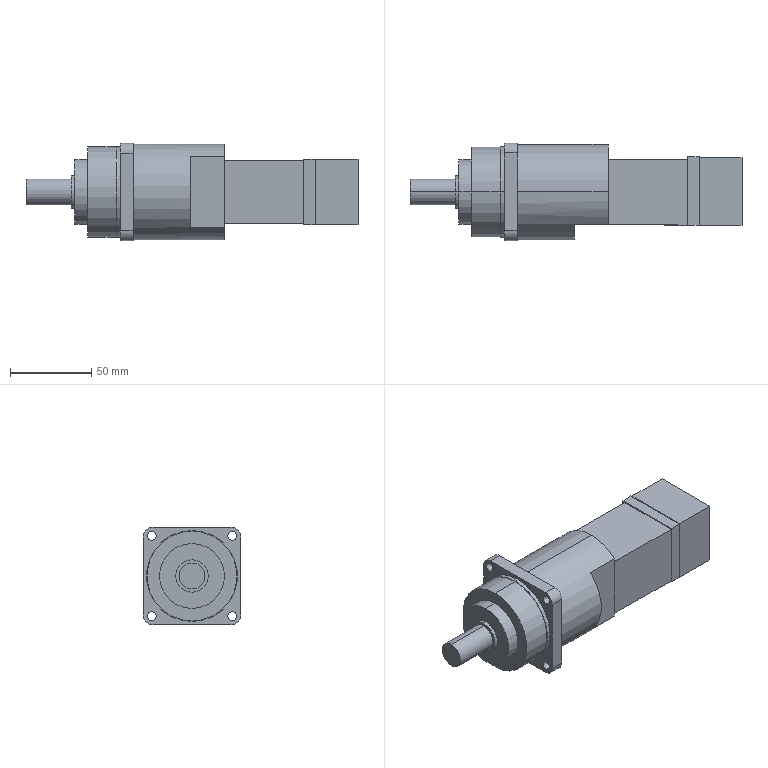Part | STEP file | 0243_102_Servo_Motor_HF-KP13G7 1_5 | 1 solid | 59 faces | box 204.4 x 60 x 60 mm | volume 372734 mm3 | plane 35 | cylinder 24 | commonest cylinder face diameters 5.5 x8 12 x4 16 x2 20 x2 40 x2 55.5 x2